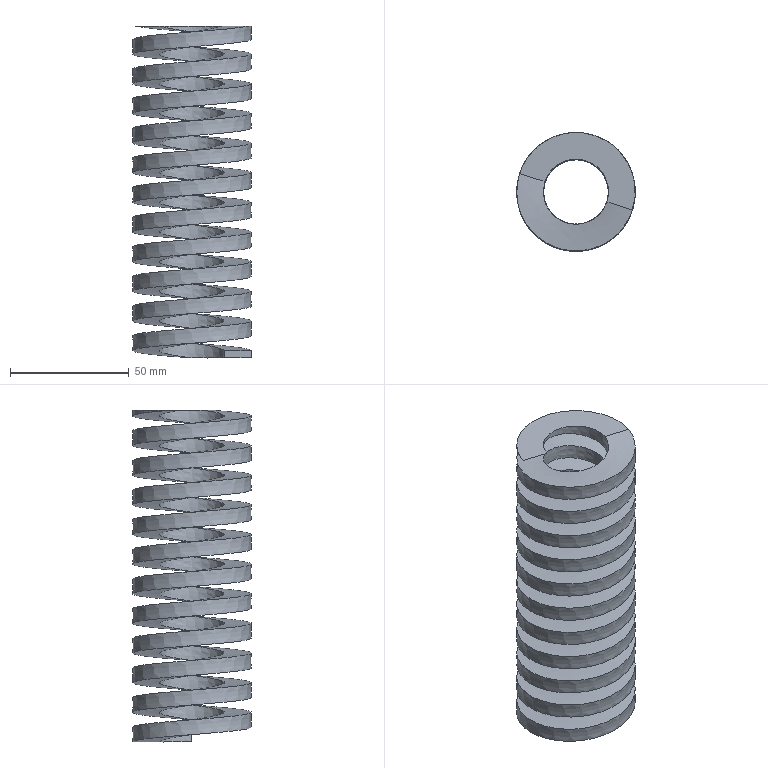Part | NX | features FTH50.00-155.00 2 | 1 solid | 7 faces | box 50 x 50 x 140 mm | volume 97410 mm3 | spline 5 | plane 2